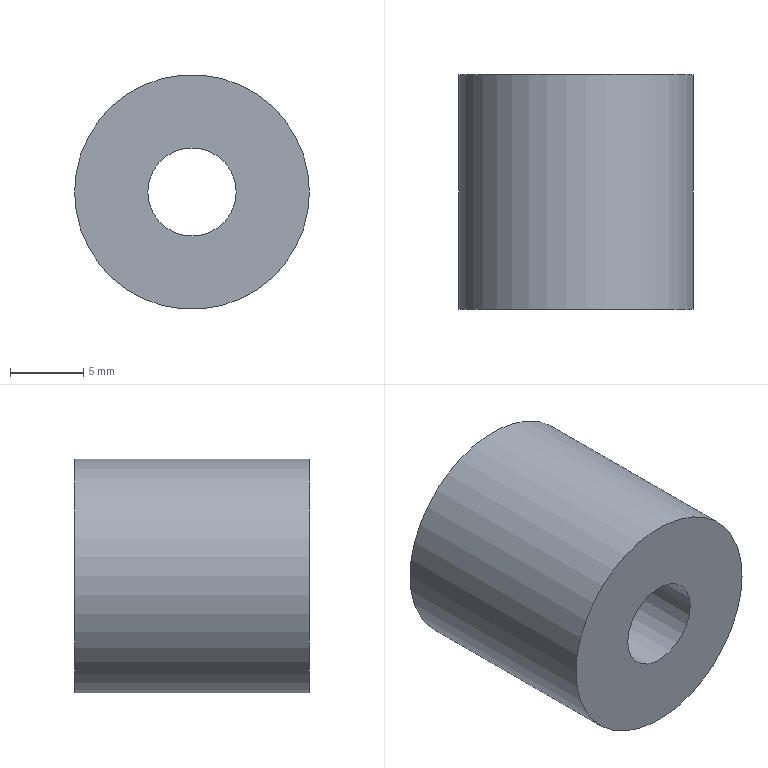Part | STEP file | 1 solid | 4 faces | box 16 x 16 x 16 mm | volume 2762 mm3 | cylinder 2 | plane 2 | commonest cylinder face diameters 6.02 x1 16 x1
STEP:
#1=CARTESIAN_POINT('',(0.,0.,0.));
#2=DIRECTION('',(0.,0.,1.));
#3=DIRECTION('',(1.,0.,0.));
#4=AXIS2_PLACEMENT_3D('',#1,#2,#3);
#5=CARTESIAN_POINT('',(1705.957,327.48,7.419));
#6=VERTEX_POINT('',#5);
#7=CARTESIAN_POINT('',(1697.957,327.48,7.419));
#8=DIRECTION('',(0.,1.,0.));
#9=DIRECTION('',(1.,0.,0.));
#10=AXIS2_PLACEMENT_3D('',#7,#8,#9);
#11=CIRCLE('',#10,8.);
#12=CARTESIAN_POINT('',(1697.957,327.48,7.419));
#13=DIRECTION('',(0.,-1.,0.));
#14=DIRECTION('',(-1.,0.,0.));
#15=AXIS2_PLACEMENT_3D('',#12,#13,#14);
#16=CYLINDRICAL_SURFACE('',#15,8.);
#17=CARTESIAN_POINT('',(9.425,0.));
#18=DIRECTION('',(-1.,0.));
#19=VECTOR('',#18,1.);
#20=LINE('',#17,#19);
#21=(GEOMETRIC_REPRESENTATION_CONTEXT(2)PARAMETRIC_REPRESENTATION_CONTEXT()REPRESENTATION_CONTEXT('',''));
#22=DEFINITIONAL_REPRESENTATION('',(#20),#21);
#23=PCURVE('',#16,#22);
#24=CARTESIAN_POINT('',(1697.957,327.48,7.419));
#25=DIRECTION('',(0.,1.,0.));
#26=DIRECTION('',(1.,0.,0.));
#27=AXIS2_PLACEMENT_3D('',#24,#25,#26);
#28=PLANE('',#27);
#29=CARTESIAN_POINT('',(0.,0.));
#30=DIRECTION('',(1.,0.));
#31=AXIS2_PLACEMENT_2D('',#29,#30);
#32=CIRCLE('',#31,8.);
#33=(GEOMETRIC_REPRESENTATION_CONTEXT(2)PARAMETRIC_REPRESENTATION_CONTEXT()REPRESENTATION_CONTEXT('',''));
#34=DEFINITIONAL_REPRESENTATION('',(#32),#33);
#35=PCURVE('',#28,#34);
#36=SURFACE_CURVE('',#11,(#23,#35),.PCURVE_S1.);
#37=EDGE_CURVE('',#6,#6,#36,.T.);
#38=ORIENTED_EDGE('',*,*,#37,.F.);
#39=CARTESIAN_POINT('',(1705.957,311.48,7.419));
#40=VERTEX_POINT('',#39);
#41=CARTESIAN_POINT('',(1705.957,327.48,7.419));
#42=CARTESIAN_POINT('',(1705.957,311.48,7.419));
#43=B_SPLINE_CURVE_WITH_KNOTS('',1,(#41,#42),.UNSPECIFIED.,.F.,.F.,(2,2),(0.,16.),.PIECEWISE_BEZIER_KNOTS.);
#44=CARTESIAN_POINT('',(9.425,0.));
#45=DIRECTION('',(0.,1.));
#46=VECTOR('',#45,1.);
#47=LINE('',#44,#46);
#48=(GEOMETRIC_REPRESENTATION_CONTEXT(2)PARAMETRIC_REPRESENTATION_CONTEXT()REPRESENTATION_CONTEXT('',''));
#49=DEFINITIONAL_REPRESENTATION('',(#47),#48);
#50=PCURVE('',#16,#49);
#51=CARTESIAN_POINT('',(3.142,0.));
#52=DIRECTION('',(0.,1.));
#53=VECTOR('',#52,1.);
#54=LINE('',#51,#53);
#55=(GEOMETRIC_REPRESENTATION_CONTEXT(2)PARAMETRIC_REPRESENTATION_CONTEXT()REPRESENTATION_CONTEXT('',''));
#56=DEFINITIONAL_REPRESENTATION('',(#54),#55);
#57=PCURVE('',#16,#56);
#58=SEAM_CURVE('',#43,(#50,#57),.PCURVE_S1.);
#59=EDGE_CURVE('',#6,#40,#58,.T.);
#60=ORIENTED_EDGE('',*,*,#59,.T.);
#61=CARTESIAN_POINT('',(1697.957,311.48,7.419));
#62=DIRECTION('',(0.,1.,0.));
#63=DIRECTION('',(1.,0.,0.));
#64=AXIS2_PLACEMENT_3D('',#61,#62,#63);
#65=CIRCLE('',#64,8.);
#66=CARTESIAN_POINT('',(9.425,16.));
#67=DIRECTION('',(-1.,0.));
#68=VECTOR('',#67,1.);
#69=LINE('',#66,#68);
#70=(GEOMETRIC_REPRESENTATION_CONTEXT(2)PARAMETRIC_REPRESENTATION_CONTEXT()REPRESENTATION_CONTEXT('',''));
#71=DEFINITIONAL_REPRESENTATION('',(#69),#70);
#72=PCURVE('',#16,#71);
#73=CARTESIAN_POINT('',(1697.957,311.48,7.419));
#74=DIRECTION('',(0.,1.,0.));
#75=DIRECTION('',(1.,0.,0.));
#76=AXIS2_PLACEMENT_3D('',#73,#74,#75);
#77=PLANE('',#76);
#78=CARTESIAN_POINT('',(0.,0.));
#79=DIRECTION('',(1.,0.));
#80=AXIS2_PLACEMENT_2D('',#78,#79);
#81=CIRCLE('',#80,8.);
#82=(GEOMETRIC_REPRESENTATION_CONTEXT(2)PARAMETRIC_REPRESENTATION_CONTEXT()REPRESENTATION_CONTEXT('',''));
#83=DEFINITIONAL_REPRESENTATION('',(#81),#82);
#84=PCURVE('',#77,#83);
#85=SURFACE_CURVE('',#65,(#72,#84),.PCURVE_S1.);
#86=EDGE_CURVE('',#40,#40,#85,.T.);
#87=ORIENTED_EDGE('',*,*,#86,.T.);
#88=ORIENTED_EDGE('',*,*,#59,.F.);
#89=EDGE_LOOP('',(#38,#60,#87,#88));
#90=FACE_BOUND('',#89,.T.);
#91=ADVANCED_FACE('',(#90),#16,.T.);
#92=CARTESIAN_POINT('',(1700.967,327.48,7.419));
#93=VERTEX_POINT('',#92);
#94=CARTESIAN_POINT('',(1697.957,327.48,7.419));
#95=DIRECTION('',(0.,-1.,0.));
#96=DIRECTION('',(1.,0.,0.));
#97=AXIS2_PLACEMENT_3D('',#94,#95,#96);
#98=CIRCLE('',#97,3.01);
#99=CARTESIAN_POINT('',(1697.957,327.48,7.419));
#100=DIRECTION('',(0.,-1.,0.));
#101=DIRECTION('',(-1.,0.,0.));
#102=AXIS2_PLACEMENT_3D('',#99,#100,#101);
#103=CYLINDRICAL_SURFACE('',#102,3.01);
#104=CARTESIAN_POINT('',(3.142,0.));
#105=DIRECTION('',(1.,0.));
#106=VECTOR('',#105,1.);
#107=LINE('',#104,#106);
#108=(GEOMETRIC_REPRESENTATION_CONTEXT(2)PARAMETRIC_REPRESENTATION_CONTEXT()REPRESENTATION_CONTEXT('',''));
#109=DEFINITIONAL_REPRESENTATION('',(#107),#108);
#110=PCURVE('',#103,#109);
#111=CARTESIAN_POINT('',(3.01,0.));
#112=CARTESIAN_POINT('',(3.01,-5.213));
#113=CARTESIAN_POINT('',(-1.505,-2.607));
#114=CARTESIAN_POINT('',(-6.02,0.));
#115=CARTESIAN_POINT('',(-1.505,2.607));
#116=CARTESIAN_POINT('',(3.01,5.213));
#117=CARTESIAN_POINT('',(3.01,0.));
#118=(BOUNDED_CURVE()B_SPLINE_CURVE(2,(#111,#112,#113,#114,#115,#116,#117),.UNSPECIFIED.,.T.,.F.)B_SPLINE_CURVE_WITH_KNOTS((1,2,2,2,2,1),(-2.094,0.,2.094,4.189,6.283,8.378),.UNSPECIFIED.)CURVE()GEOMETRIC_REPRESENTATION_ITEM()RATIONAL_B_SPLINE_CURVE((1.,0.5,1.,0.5,1.,0.5,1.))REPRESENTATION_ITEM(''));
#119=(GEOMETRIC_REPRESENTATION_CONTEXT(2)PARAMETRIC_REPRESENTATION_CONTEXT()REPRESENTATION_CONTEXT('',''));
#120=DEFINITIONAL_REPRESENTATION('',(#118),#119);
#121=PCURVE('',#28,#120);
#122=SURFACE_CURVE('',#98,(#110,#121),.PCURVE_S1.);
#123=EDGE_CURVE('',#93,#93,#122,.T.);
#124=ORIENTED_EDGE('',*,*,#123,.T.);
#125=CARTESIAN_POINT('',(1700.967,311.48,7.419));
#126=VERTEX_POINT('',#125);
#127=CARTESIAN_POINT('',(1700.967,327.48,7.419));
#128=CARTESIAN_POINT('',(1700.967,311.48,7.419));
#129=B_SPLINE_CURVE_WITH_KNOTS('',1,(#127,#128),.UNSPECIFIED.,.F.,.F.,(2,2),(0.,16.),.PIECEWISE_BEZIER_KNOTS.);
#130=CARTESIAN_POINT('',(9.425,0.));
#131=DIRECTION('',(0.,1.));
#132=VECTOR('',#131,1.);
#133=LINE('',#130,#132);
#134=(GEOMETRIC_REPRESENTATION_CONTEXT(2)PARAMETRIC_REPRESENTATION_CONTEXT()REPRESENTATION_CONTEXT('',''));
#135=DEFINITIONAL_REPRESENTATION('',(#133),#134);
#136=PCURVE('',#103,#135);
#137=CARTESIAN_POINT('',(3.142,0.));
#138=DIRECTION('',(0.,1.));
#139=VECTOR('',#138,1.);
#140=LINE('',#137,#139);
#141=(GEOMETRIC_REPRESENTATION_CONTEXT(2)PARAMETRIC_REPRESENTATION_CONTEXT()REPRESENTATION_CONTEXT('',''));
#142=DEFINITIONAL_REPRESENTATION('',(#140),#141);
#143=PCURVE('',#103,#142);
#144=SEAM_CURVE('',#129,(#136,#143),.PCURVE_S1.);
#145=EDGE_CURVE('',#93,#126,#144,.T.);
#146=ORIENTED_EDGE('',*,*,#145,.T.);
#147=CARTESIAN_POINT('',(1697.957,311.48,7.419));
#148=DIRECTION('',(0.,-1.,0.));
#149=DIRECTION('',(1.,0.,0.));
#150=AXIS2_PLACEMENT_3D('',#147,#148,#149);
#151=CIRCLE('',#150,3.01);
#152=CARTESIAN_POINT('',(3.142,16.));
#153=DIRECTION('',(1.,0.));
#154=VECTOR('',#153,1.);
#155=LINE('',#152,#154);
#156=(GEOMETRIC_REPRESENTATION_CONTEXT(2)PARAMETRIC_REPRESENTATION_CONTEXT()REPRESENTATION_CONTEXT('',''));
#157=DEFINITIONAL_REPRESENTATION('',(#155),#156);
#158=PCURVE('',#103,#157);
#159=CARTESIAN_POINT('',(3.01,0.));
#160=CARTESIAN_POINT('',(3.01,-5.213));
#161=CARTESIAN_POINT('',(-1.505,-2.607));
#162=CARTESIAN_POINT('',(-6.02,0.));
#163=CARTESIAN_POINT('',(-1.505,2.607));
#164=CARTESIAN_POINT('',(3.01,5.213));
#165=CARTESIAN_POINT('',(3.01,0.));
#166=(BOUNDED_CURVE()B_SPLINE_CURVE(2,(#159,#160,#161,#162,#163,#164,#165),.UNSPECIFIED.,.T.,.F.)B_SPLINE_CURVE_WITH_KNOTS((1,2,2,2,2,1),(-2.094,0.,2.094,4.189,6.283,8.378),.UNSPECIFIED.)CURVE()GEOMETRIC_REPRESENTATION_ITEM()RATIONAL_B_SPLINE_CURVE((1.,0.5,1.,0.5,1.,0.5,1.))REPRESENTATION_ITEM(''));
#167=(GEOMETRIC_REPRESENTATION_CONTEXT(2)PARAMETRIC_REPRESENTATION_CONTEXT()REPRESENTATION_CONTEXT('',''));
#168=DEFINITIONAL_REPRESENTATION('',(#166),#167);
#169=PCURVE('',#77,#168);
#170=SURFACE_CURVE('',#151,(#158,#169),.PCURVE_S1.);
#171=EDGE_CURVE('',#126,#126,#170,.T.);
#172=ORIENTED_EDGE('',*,*,#171,.F.);
#173=ORIENTED_EDGE('',*,*,#145,.F.);
#174=EDGE_LOOP('',(#124,#146,#172,#173));
#175=FACE_BOUND('',#174,.F.);
#176=ADVANCED_FACE('',(#175),#103,.F.);
#177=ORIENTED_EDGE('',*,*,#37,.T.);
#178=EDGE_LOOP('',(#177));
#179=FACE_BOUND('',#178,.T.);
#180=ORIENTED_EDGE('',*,*,#123,.T.);
#181=EDGE_LOOP('',(#180));
#182=FACE_BOUND('',#181,.T.);
#183=ADVANCED_FACE('',(#179,#182),#28,.T.);
#184=ORIENTED_EDGE('',*,*,#86,.F.);
#185=EDGE_LOOP('',(#184));
#186=FACE_BOUND('',#185,.T.);
#187=ORIENTED_EDGE('',*,*,#171,.F.);
#188=EDGE_LOOP('',(#187));
#189=FACE_BOUND('',#188,.T.);
#190=ADVANCED_FACE('',(#186,#189),#77,.F.);
#191=CLOSED_SHELL('',(#91,#176,#183,#190));
#192=MANIFOLD_SOLID_BREP('',#191);
#193=(LENGTH_UNIT()NAMED_UNIT(*)SI_UNIT(.MILLI.,.METRE.));
#194=UNCERTAINTY_MEASURE_WITH_UNIT(LENGTH_MEASURE(0.00001),#193,'','');
#195=(NAMED_UNIT(*)PLANE_ANGLE_UNIT()SI_UNIT($,.RADIAN.));
#196=(NAMED_UNIT(*)SI_UNIT($,.STERADIAN.)SOLID_ANGLE_UNIT());
#197=(GEOMETRIC_REPRESENTATION_CONTEXT(3)GLOBAL_UNCERTAINTY_ASSIGNED_CONTEXT((#194))GLOBAL_UNIT_ASSIGNED_CONTEXT((#193,#195,#196))REPRESENTATION_CONTEXT('',''));
#198=ADVANCED_BREP_SHAPE_REPRESENTATION('',(#4,#192),#197);